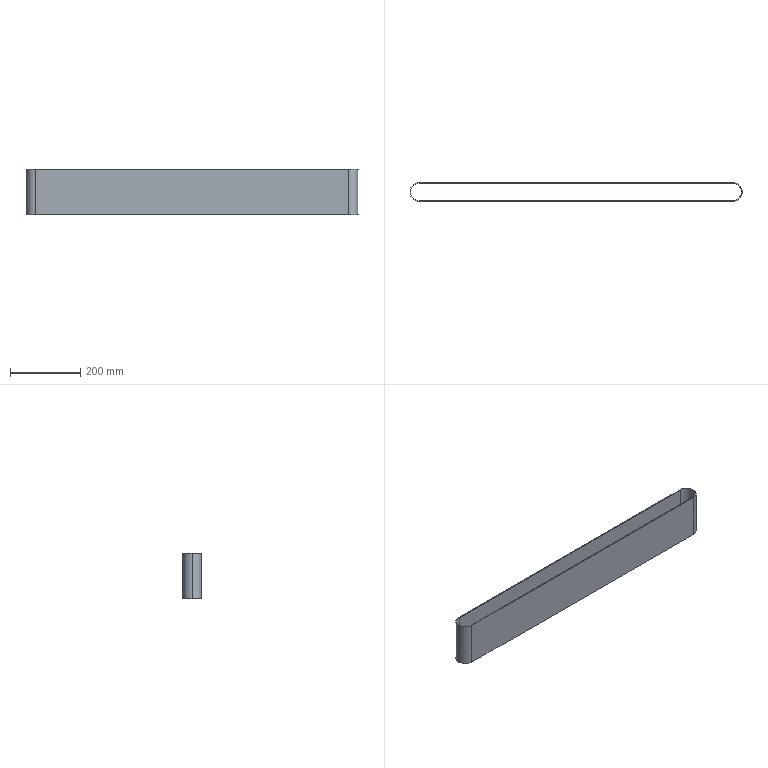Part | STEP file | Light green PVC conveyor belt 1946x129x2mm thick_antistatic | 1 solid | 12 faces | box 948.5 x 54 x 129 mm | volume 503710 mm3 | cylinder 6 | plane 6 | commonest cylinder face diameters 50 x3 54 x3
STEP:
#1=CARTESIAN_POINT('',(0.,0.,0.));
#2=DIRECTION('',(0.,0.,1.));
#3=DIRECTION('',(1.,0.,0.));
#4=AXIS2_PLACEMENT_3D('',#1,#2,#3);
#5=CARTESIAN_POINT('',(-447.25,25.,64.5));
#6=VERTEX_POINT('',#5);
#7=CARTESIAN_POINT('',(-447.25,25.,-64.5));
#8=VERTEX_POINT('',#7);
#9=CARTESIAN_POINT('',(-447.25,25.,64.5));
#10=DIRECTION('',(0.,0.,-1.));
#11=VECTOR('',#10,1.);
#12=LINE('',#9,#11);
#13=CARTESIAN_POINT('',(-447.25,0.,64.5));
#14=DIRECTION('',(0.,0.,-1.));
#15=DIRECTION('',(-1.,0.,0.));
#16=AXIS2_PLACEMENT_3D('',#13,#14,#15);
#17=CYLINDRICAL_SURFACE('',#16,25.);
#18=CARTESIAN_POINT('',(1.571,0.));
#19=DIRECTION('',(0.,1.));
#20=VECTOR('',#19,1.);
#21=LINE('',#18,#20);
#22=(GEOMETRIC_REPRESENTATION_CONTEXT(2)PARAMETRIC_REPRESENTATION_CONTEXT()REPRESENTATION_CONTEXT('',''));
#23=DEFINITIONAL_REPRESENTATION('',(#21),#22);
#24=PCURVE('',#17,#23);
#25=CARTESIAN_POINT('',(-447.25,25.,64.5));
#26=DIRECTION('',(0.,-1.,0.));
#27=DIRECTION('',(0.,0.,-1.));
#28=AXIS2_PLACEMENT_3D('',#25,#26,#27);
#29=PLANE('',#28);
#30=CARTESIAN_POINT('',(0.,0.));
#31=DIRECTION('',(1.,0.));
#32=VECTOR('',#31,1.);
#33=LINE('',#30,#32);
#34=(GEOMETRIC_REPRESENTATION_CONTEXT(2)PARAMETRIC_REPRESENTATION_CONTEXT()REPRESENTATION_CONTEXT('',''));
#35=DEFINITIONAL_REPRESENTATION('',(#33),#34);
#36=PCURVE('',#29,#35);
#37=SURFACE_CURVE('',#12,(#24,#36),.PCURVE_S1.);
#38=EDGE_CURVE('',#6,#8,#37,.T.);
#39=ORIENTED_EDGE('',*,*,#38,.T.);
#40=CARTESIAN_POINT('',(-472.25,0.,-64.5));
#41=VERTEX_POINT('',#40);
#42=CARTESIAN_POINT('',(-447.25,0.,-64.5));
#43=DIRECTION('',(0.,0.,1.));
#44=DIRECTION('',(1.,0.,0.));
#45=AXIS2_PLACEMENT_3D('',#42,#43,#44);
#46=CIRCLE('',#45,25.);
#47=CARTESIAN_POINT('',(3.142,129.));
#48=DIRECTION('',(-1.,0.));
#49=VECTOR('',#48,1.);
#50=LINE('',#47,#49);
#51=(GEOMETRIC_REPRESENTATION_CONTEXT(2)PARAMETRIC_REPRESENTATION_CONTEXT()REPRESENTATION_CONTEXT('',''));
#52=DEFINITIONAL_REPRESENTATION('',(#50),#51);
#53=PCURVE('',#17,#52);
#54=CARTESIAN_POINT('',(-447.25,0.,-64.5));
#55=DIRECTION('',(0.,0.,1.));
#56=DIRECTION('',(1.,0.,0.));
#57=AXIS2_PLACEMENT_3D('',#54,#55,#56);
#58=PLANE('',#57);
#59=CARTESIAN_POINT('',(0.,0.));
#60=DIRECTION('',(1.,0.));
#61=AXIS2_PLACEMENT_2D('',#59,#60);
#62=CIRCLE('',#61,25.);
#63=(GEOMETRIC_REPRESENTATION_CONTEXT(2)PARAMETRIC_REPRESENTATION_CONTEXT()REPRESENTATION_CONTEXT('',''));
#64=DEFINITIONAL_REPRESENTATION('',(#62),#63);
#65=PCURVE('',#58,#64);
#66=SURFACE_CURVE('',#46,(#53,#65),.PCURVE_S1.);
#67=EDGE_CURVE('',#8,#41,#66,.T.);
#68=ORIENTED_EDGE('',*,*,#67,.T.);
#69=CARTESIAN_POINT('',(-472.25,0.,64.5));
#70=VERTEX_POINT('',#69);
#71=CARTESIAN_POINT('',(-472.25,0.,64.5));
#72=DIRECTION('',(0.,0.,-1.));
#73=VECTOR('',#72,1.);
#74=LINE('',#71,#73);
#75=CARTESIAN_POINT('',(0.,0.));
#76=DIRECTION('',(0.,1.));
#77=VECTOR('',#76,1.);
#78=LINE('',#75,#77);
#79=(GEOMETRIC_REPRESENTATION_CONTEXT(2)PARAMETRIC_REPRESENTATION_CONTEXT()REPRESENTATION_CONTEXT('',''));
#80=DEFINITIONAL_REPRESENTATION('',(#78),#79);
#81=PCURVE('',#17,#80);
#82=CARTESIAN_POINT('',(-447.25,0.,64.5));
#83=DIRECTION('',(0.,0.,-1.));
#84=DIRECTION('',(-1.,0.,0.));
#85=AXIS2_PLACEMENT_3D('',#82,#83,#84);
#86=CYLINDRICAL_SURFACE('',#85,25.);
#87=CARTESIAN_POINT('',(6.283,0.));
#88=DIRECTION('',(0.,1.));
#89=VECTOR('',#88,1.);
#90=LINE('',#87,#89);
#91=(GEOMETRIC_REPRESENTATION_CONTEXT(2)PARAMETRIC_REPRESENTATION_CONTEXT()REPRESENTATION_CONTEXT('',''));
#92=DEFINITIONAL_REPRESENTATION('',(#90),#91);
#93=PCURVE('',#86,#92);
#94=SURFACE_CURVE('',#74,(#81,#93),.PCURVE_S1.);
#95=EDGE_CURVE('',#70,#41,#94,.T.);
#96=ORIENTED_EDGE('',*,*,#95,.F.);
#97=CARTESIAN_POINT('',(-447.25,0.,64.5));
#98=DIRECTION('',(0.,0.,1.));
#99=DIRECTION('',(1.,0.,0.));
#100=AXIS2_PLACEMENT_3D('',#97,#98,#99);
#101=CIRCLE('',#100,25.);
#102=CARTESIAN_POINT('',(3.142,0.));
#103=DIRECTION('',(-1.,0.));
#104=VECTOR('',#103,1.);
#105=LINE('',#102,#104);
#106=(GEOMETRIC_REPRESENTATION_CONTEXT(2)PARAMETRIC_REPRESENTATION_CONTEXT()REPRESENTATION_CONTEXT('',''));
#107=DEFINITIONAL_REPRESENTATION('',(#105),#106);
#108=PCURVE('',#17,#107);
#109=CARTESIAN_POINT('',(-447.25,0.,64.5));
#110=DIRECTION('',(0.,0.,1.));
#111=DIRECTION('',(1.,0.,0.));
#112=AXIS2_PLACEMENT_3D('',#109,#110,#111);
#113=PLANE('',#112);
#114=CARTESIAN_POINT('',(0.,0.));
#115=DIRECTION('',(1.,0.));
#116=AXIS2_PLACEMENT_2D('',#114,#115);
#117=CIRCLE('',#116,25.);
#118=(GEOMETRIC_REPRESENTATION_CONTEXT(2)PARAMETRIC_REPRESENTATION_CONTEXT()REPRESENTATION_CONTEXT('',''));
#119=DEFINITIONAL_REPRESENTATION('',(#117),#118);
#120=PCURVE('',#113,#119);
#121=SURFACE_CURVE('',#101,(#108,#120),.PCURVE_S1.);
#122=EDGE_CURVE('',#6,#70,#121,.T.);
#123=ORIENTED_EDGE('',*,*,#122,.F.);
#124=EDGE_LOOP('',(#39,#68,#96,#123));
#125=FACE_BOUND('',#124,.F.);
#126=ADVANCED_FACE('',(#125),#17,.F.);
#127=CARTESIAN_POINT('',(-474.25,0.,64.5));
#128=VERTEX_POINT('',#127);
#129=CARTESIAN_POINT('',(-447.25,-27.,64.5));
#130=VERTEX_POINT('',#129);
#131=CARTESIAN_POINT('',(-447.25,0.,64.5));
#132=DIRECTION('',(0.,0.,1.));
#133=DIRECTION('',(1.,0.,0.));
#134=AXIS2_PLACEMENT_3D('',#131,#132,#133);
#135=CIRCLE('',#134,27.);
#136=CARTESIAN_POINT('',(-447.25,0.,64.5));
#137=DIRECTION('',(0.,0.,-1.));
#138=DIRECTION('',(-1.,0.,0.));
#139=AXIS2_PLACEMENT_3D('',#136,#137,#138);
#140=CYLINDRICAL_SURFACE('',#139,27.);
#141=CARTESIAN_POINT('',(9.425,0.));
#142=DIRECTION('',(-1.,0.));
#143=VECTOR('',#142,1.);
#144=LINE('',#141,#143);
#145=(GEOMETRIC_REPRESENTATION_CONTEXT(2)PARAMETRIC_REPRESENTATION_CONTEXT()REPRESENTATION_CONTEXT('',''));
#146=DEFINITIONAL_REPRESENTATION('',(#144),#145);
#147=PCURVE('',#140,#146);
#148=CARTESIAN_POINT('',(0.,0.));
#149=DIRECTION('',(1.,0.));
#150=AXIS2_PLACEMENT_2D('',#148,#149);
#151=CIRCLE('',#150,27.);
#152=(GEOMETRIC_REPRESENTATION_CONTEXT(2)PARAMETRIC_REPRESENTATION_CONTEXT()REPRESENTATION_CONTEXT('',''));
#153=DEFINITIONAL_REPRESENTATION('',(#151),#152);
#154=PCURVE('',#113,#153);
#155=SURFACE_CURVE('',#135,(#147,#154),.PCURVE_S1.);
#156=EDGE_CURVE('',#128,#130,#155,.T.);
#157=ORIENTED_EDGE('',*,*,#156,.F.);
#158=CARTESIAN_POINT('',(-474.25,0.,-64.5));
#159=VERTEX_POINT('',#158);
#160=CARTESIAN_POINT('',(-474.25,0.,64.5));
#161=DIRECTION('',(0.,0.,-1.));
#162=VECTOR('',#161,1.);
#163=LINE('',#160,#162);
#164=CARTESIAN_POINT('',(6.283,0.));
#165=DIRECTION('',(0.,1.));
#166=VECTOR('',#165,1.);
#167=LINE('',#164,#166);
#168=(GEOMETRIC_REPRESENTATION_CONTEXT(2)PARAMETRIC_REPRESENTATION_CONTEXT()REPRESENTATION_CONTEXT('',''));
#169=DEFINITIONAL_REPRESENTATION('',(#167),#168);
#170=PCURVE('',#140,#169);
#171=CARTESIAN_POINT('',(-447.25,0.,64.5));
#172=DIRECTION('',(0.,0.,-1.));
#173=DIRECTION('',(-1.,0.,0.));
#174=AXIS2_PLACEMENT_3D('',#171,#172,#173);
#175=CYLINDRICAL_SURFACE('',#174,27.);
#176=CARTESIAN_POINT('',(0.,0.));
#177=DIRECTION('',(0.,1.));
#178=VECTOR('',#177,1.);
#179=LINE('',#176,#178);
#180=(GEOMETRIC_REPRESENTATION_CONTEXT(2)PARAMETRIC_REPRESENTATION_CONTEXT()REPRESENTATION_CONTEXT('',''));
#181=DEFINITIONAL_REPRESENTATION('',(#179),#180);
#182=PCURVE('',#175,#181);
#183=SURFACE_CURVE('',#163,(#170,#182),.PCURVE_S1.);
#184=EDGE_CURVE('',#128,#159,#183,.T.);
#185=ORIENTED_EDGE('',*,*,#184,.T.);
#186=CARTESIAN_POINT('',(-447.25,-27.,-64.5));
#187=VERTEX_POINT('',#186);
#188=CARTESIAN_POINT('',(-447.25,0.,-64.5));
#189=DIRECTION('',(0.,0.,1.));
#190=DIRECTION('',(1.,0.,0.));
#191=AXIS2_PLACEMENT_3D('',#188,#189,#190);
#192=CIRCLE('',#191,27.);
#193=CARTESIAN_POINT('',(9.425,129.));
#194=DIRECTION('',(-1.,0.));
#195=VECTOR('',#194,1.);
#196=LINE('',#193,#195);
#197=(GEOMETRIC_REPRESENTATION_CONTEXT(2)PARAMETRIC_REPRESENTATION_CONTEXT()REPRESENTATION_CONTEXT('',''));
#198=DEFINITIONAL_REPRESENTATION('',(#196),#197);
#199=PCURVE('',#140,#198);
#200=CARTESIAN_POINT('',(0.,0.));
#201=DIRECTION('',(1.,0.));
#202=AXIS2_PLACEMENT_2D('',#200,#201);
#203=CIRCLE('',#202,27.);
#204=(GEOMETRIC_REPRESENTATION_CONTEXT(2)PARAMETRIC_REPRESENTATION_CONTEXT()REPRESENTATION_CONTEXT('',''));
#205=DEFINITIONAL_REPRESENTATION('',(#203),#204);
#206=PCURVE('',#58,#205);
#207=SURFACE_CURVE('',#192,(#199,#206),.PCURVE_S1.);
#208=EDGE_CURVE('',#159,#187,#207,.T.);
#209=ORIENTED_EDGE('',*,*,#208,.T.);
#210=CARTESIAN_POINT('',(-447.25,-27.,64.5));
#211=DIRECTION('',(0.,0.,-1.));
#212=VECTOR('',#211,1.);
#213=LINE('',#210,#212);
#214=CARTESIAN_POINT('',(4.712,0.));
#215=DIRECTION('',(0.,1.));
#216=VECTOR('',#215,1.);
#217=LINE('',#214,#216);
#218=(GEOMETRIC_REPRESENTATION_CONTEXT(2)PARAMETRIC_REPRESENTATION_CONTEXT()REPRESENTATION_CONTEXT('',''));
#219=DEFINITIONAL_REPRESENTATION('',(#217),#218);
#220=PCURVE('',#140,#219);
#221=CARTESIAN_POINT('',(-447.25,-27.,64.5));
#222=DIRECTION('',(0.,1.,0.));
#223=DIRECTION('',(0.,0.,1.));
#224=AXIS2_PLACEMENT_3D('',#221,#222,#223);
#225=PLANE('',#224);
#226=CARTESIAN_POINT('',(0.,0.));
#227=DIRECTION('',(-1.,0.));
#228=VECTOR('',#227,1.);
#229=LINE('',#226,#228);
#230=(GEOMETRIC_REPRESENTATION_CONTEXT(2)PARAMETRIC_REPRESENTATION_CONTEXT()REPRESENTATION_CONTEXT('',''));
#231=DEFINITIONAL_REPRESENTATION('',(#229),#230);
#232=PCURVE('',#225,#231);
#233=SURFACE_CURVE('',#213,(#220,#232),.PCURVE_S1.);
#234=EDGE_CURVE('',#130,#187,#233,.T.);
#235=ORIENTED_EDGE('',*,*,#234,.F.);
#236=EDGE_LOOP('',(#157,#185,#209,#235));
#237=FACE_BOUND('',#236,.T.);
#238=ADVANCED_FACE('',(#237),#140,.T.);
#239=CARTESIAN_POINT('',(-447.25,27.,64.5));
#240=VERTEX_POINT('',#239);
#241=CARTESIAN_POINT('',(-447.25,0.,64.5));
#242=DIRECTION('',(0.,0.,1.));
#243=DIRECTION('',(1.,0.,0.));
#244=AXIS2_PLACEMENT_3D('',#241,#242,#243);
#245=CIRCLE('',#244,27.);
#246=CARTESIAN_POINT('',(0.,0.));
#247=DIRECTION('',(1.,0.));
#248=AXIS2_PLACEMENT_2D('',#246,#247);
#249=CIRCLE('',#248,27.);
#250=(GEOMETRIC_REPRESENTATION_CONTEXT(2)PARAMETRIC_REPRESENTATION_CONTEXT()REPRESENTATION_CONTEXT('',''));
#251=DEFINITIONAL_REPRESENTATION('',(#249),#250);
#252=PCURVE('',#113,#251);
#253=CARTESIAN_POINT('',(3.142,0.));
#254=DIRECTION('',(-1.,0.));
#255=VECTOR('',#254,1.);
#256=LINE('',#253,#255);
#257=(GEOMETRIC_REPRESENTATION_CONTEXT(2)PARAMETRIC_REPRESENTATION_CONTEXT()REPRESENTATION_CONTEXT('',''));
#258=DEFINITIONAL_REPRESENTATION('',(#256),#257);
#259=PCURVE('',#175,#258);
#260=SURFACE_CURVE('',#245,(#252,#259),.PCURVE_S1.);
#261=EDGE_CURVE('',#240,#128,#260,.T.);
#262=ORIENTED_EDGE('',*,*,#261,.T.);
#263=ORIENTED_EDGE('',*,*,#156,.T.);
#264=CARTESIAN_POINT('',(447.25,-27.,64.5));
#265=VERTEX_POINT('',#264);
#266=CARTESIAN_POINT('',(-447.25,-27.,64.5));
#267=DIRECTION('',(1.,0.,0.));
#268=VECTOR('',#267,1.);
#269=LINE('',#266,#268);
#270=CARTESIAN_POINT('',(0.,-27.));
#271=DIRECTION('',(1.,0.));
#272=VECTOR('',#271,1.);
#273=LINE('',#270,#272);
#274=(GEOMETRIC_REPRESENTATION_CONTEXT(2)PARAMETRIC_REPRESENTATION_CONTEXT()REPRESENTATION_CONTEXT('',''));
#275=DEFINITIONAL_REPRESENTATION('',(#273),#274);
#276=PCURVE('',#113,#275);
#277=CARTESIAN_POINT('',(0.,0.));
#278=DIRECTION('',(0.,1.));
#279=VECTOR('',#278,1.);
#280=LINE('',#277,#279);
#281=(GEOMETRIC_REPRESENTATION_CONTEXT(2)PARAMETRIC_REPRESENTATION_CONTEXT()REPRESENTATION_CONTEXT('',''));
#282=DEFINITIONAL_REPRESENTATION('',(#280),#281);
#283=PCURVE('',#225,#282);
#284=SURFACE_CURVE('',#269,(#276,#283),.PCURVE_S1.);
#285=EDGE_CURVE('',#130,#265,#284,.T.);
#286=ORIENTED_EDGE('',*,*,#285,.T.);
#287=CARTESIAN_POINT('',(447.25,27.,64.5));
#288=VERTEX_POINT('',#287);
#289=CARTESIAN_POINT('',(447.25,0.,64.5));
#290=DIRECTION('',(0.,0.,1.));
#291=DIRECTION('',(1.,0.,0.));
#292=AXIS2_PLACEMENT_3D('',#289,#290,#291);
#293=CIRCLE('',#292,27.);
#294=CARTESIAN_POINT('',(894.5,0.));
#295=DIRECTION('',(1.,0.));
#296=AXIS2_PLACEMENT_2D('',#294,#295);
#297=CIRCLE('',#296,27.);
#298=(GEOMETRIC_REPRESENTATION_CONTEXT(2)PARAMETRIC_REPRESENTATION_CONTEXT()REPRESENTATION_CONTEXT('',''));
#299=DEFINITIONAL_REPRESENTATION('',(#297),#298);
#300=PCURVE('',#113,#299);
#301=CARTESIAN_POINT('',(447.25,0.,64.5));
#302=DIRECTION('',(0.,0.,-1.));
#303=DIRECTION('',(-1.,0.,0.));
#304=AXIS2_PLACEMENT_3D('',#301,#302,#303);
#305=CYLINDRICAL_SURFACE('',#304,27.);
#306=CARTESIAN_POINT('',(9.425,0.));
#307=DIRECTION('',(-1.,0.));
#308=VECTOR('',#307,1.);
#309=LINE('',#306,#308);
#310=(GEOMETRIC_REPRESENTATION_CONTEXT(2)PARAMETRIC_REPRESENTATION_CONTEXT()REPRESENTATION_CONTEXT('',''));
#311=DEFINITIONAL_REPRESENTATION('',(#309),#310);
#312=PCURVE('',#305,#311);
#313=SURFACE_CURVE('',#293,(#300,#312),.PCURVE_S1.);
#314=EDGE_CURVE('',#265,#288,#313,.T.);
#315=ORIENTED_EDGE('',*,*,#314,.T.);
#316=CARTESIAN_POINT('',(-447.25,27.,64.5));
#317=DIRECTION('',(-1.,0.,0.));
#318=VECTOR('',#317,1.);
#319=LINE('',#316,#318);
#320=CARTESIAN_POINT('',(0.,27.));
#321=DIRECTION('',(-1.,0.));
#322=VECTOR('',#321,1.);
#323=LINE('',#320,#322);
#324=(GEOMETRIC_REPRESENTATION_CONTEXT(2)PARAMETRIC_REPRESENTATION_CONTEXT()REPRESENTATION_CONTEXT('',''));
#325=DEFINITIONAL_REPRESENTATION('',(#323),#324);
#326=PCURVE('',#113,#325);
#327=CARTESIAN_POINT('',(-447.25,27.,64.5));
#328=DIRECTION('',(0.,-1.,0.));
#329=DIRECTION('',(0.,0.,-1.));
#330=AXIS2_PLACEMENT_3D('',#327,#328,#329);
#331=PLANE('',#330);
#332=CARTESIAN_POINT('',(0.,0.));
#333=DIRECTION('',(0.,-1.));
#334=VECTOR('',#333,1.);
#335=LINE('',#332,#334);
#336=(GEOMETRIC_REPRESENTATION_CONTEXT(2)PARAMETRIC_REPRESENTATION_CONTEXT()REPRESENTATION_CONTEXT('',''));
#337=DEFINITIONAL_REPRESENTATION('',(#335),#336);
#338=PCURVE('',#331,#337);
#339=SURFACE_CURVE('',#319,(#326,#338),.PCURVE_S1.);
#340=EDGE_CURVE('',#288,#240,#339,.T.);
#341=ORIENTED_EDGE('',*,*,#340,.T.);
#342=EDGE_LOOP('',(#262,#263,#286,#315,#341));
#343=FACE_BOUND('',#342,.T.);
#344=CARTESIAN_POINT('',(-447.25,-25.,64.5));
#345=VERTEX_POINT('',#344);
#346=CARTESIAN_POINT('',(447.25,-25.,64.5));
#347=VERTEX_POINT('',#346);
#348=CARTESIAN_POINT('',(-447.25,-25.,64.5));
#349=DIRECTION('',(1.,0.,0.));
#350=VECTOR('',#349,1.);
#351=LINE('',#348,#350);
#352=CARTESIAN_POINT('',(0.,-25.));
#353=DIRECTION('',(1.,0.));
#354=VECTOR('',#353,1.);
#355=LINE('',#352,#354);
#356=(GEOMETRIC_REPRESENTATION_CONTEXT(2)PARAMETRIC_REPRESENTATION_CONTEXT()REPRESENTATION_CONTEXT('',''));
#357=DEFINITIONAL_REPRESENTATION('',(#355),#356);
#358=PCURVE('',#113,#357);
#359=CARTESIAN_POINT('',(-447.25,-25.,64.5));
#360=DIRECTION('',(0.,1.,0.));
#361=DIRECTION('',(0.,0.,1.));
#362=AXIS2_PLACEMENT_3D('',#359,#360,#361);
#363=PLANE('',#362);
#364=CARTESIAN_POINT('',(0.,0.));
#365=DIRECTION('',(0.,1.));
#366=VECTOR('',#365,1.);
#367=LINE('',#364,#366);
#368=(GEOMETRIC_REPRESENTATION_CONTEXT(2)PARAMETRIC_REPRESENTATION_CONTEXT()REPRESENTATION_CONTEXT('',''));
#369=DEFINITIONAL_REPRESENTATION('',(#367),#368);
#370=PCURVE('',#363,#369);
#371=SURFACE_CURVE('',#351,(#358,#370),.PCURVE_S1.);
#372=EDGE_CURVE('',#345,#347,#371,.T.);
#373=ORIENTED_EDGE('',*,*,#372,.F.);
#374=CARTESIAN_POINT('',(-447.25,0.,64.5));
#375=DIRECTION('',(0.,0.,1.));
#376=DIRECTION('',(1.,0.,0.));
#377=AXIS2_PLACEMENT_3D('',#374,#375,#376);
#378=CIRCLE('',#377,25.);
#379=CARTESIAN_POINT('',(0.,0.));
#380=DIRECTION('',(1.,0.));
#381=AXIS2_PLACEMENT_2D('',#379,#380);
#382=CIRCLE('',#381,25.);
#383=(GEOMETRIC_REPRESENTATION_CONTEXT(2)PARAMETRIC_REPRESENTATION_CONTEXT()REPRESENTATION_CONTEXT('',''));
#384=DEFINITIONAL_REPRESENTATION('',(#382),#383);
#385=PCURVE('',#113,#384);
#386=CARTESIAN_POINT('',(9.425,0.));
#387=DIRECTION('',(-1.,0.));
#388=VECTOR('',#387,1.);
#389=LINE('',#386,#388);
#390=(GEOMETRIC_REPRESENTATION_CONTEXT(2)PARAMETRIC_REPRESENTATION_CONTEXT()REPRESENTATION_CONTEXT('',''));
#391=DEFINITIONAL_REPRESENTATION('',(#389),#390);
#392=PCURVE('',#86,#391);
#393=SURFACE_CURVE('',#378,(#385,#392),.PCURVE_S1.);
#394=EDGE_CURVE('',#70,#345,#393,.T.);
#395=ORIENTED_EDGE('',*,*,#394,.F.);
#396=ORIENTED_EDGE('',*,*,#122,.F.);
#397=CARTESIAN_POINT('',(447.25,25.,64.5));
#398=VERTEX_POINT('',#397);
#399=CARTESIAN_POINT('',(-447.25,25.,64.5));
#400=DIRECTION('',(-1.,0.,0.));
#401=VECTOR('',#400,1.);
#402=LINE('',#399,#401);
#403=CARTESIAN_POINT('',(0.,25.));
#404=DIRECTION('',(-1.,0.));
#405=VECTOR('',#404,1.);
#406=LINE('',#403,#405);
#407=(GEOMETRIC_REPRESENTATION_CONTEXT(2)PARAMETRIC_REPRESENTATION_CONTEXT()REPRESENTATION_CONTEXT('',''));
#408=DEFINITIONAL_REPRESENTATION('',(#406),#407);
#409=PCURVE('',#113,#408);
#410=CARTESIAN_POINT('',(0.,0.));
#411=DIRECTION('',(0.,-1.));
#412=VECTOR('',#411,1.);
#413=LINE('',#410,#412);
#414=(GEOMETRIC_REPRESENTATION_CONTEXT(2)PARAMETRIC_REPRESENTATION_CONTEXT()REPRESENTATION_CONTEXT('',''));
#415=DEFINITIONAL_REPRESENTATION('',(#413),#414);
#416=PCURVE('',#29,#415);
#417=SURFACE_CURVE('',#402,(#409,#416),.PCURVE_S1.);
#418=EDGE_CURVE('',#398,#6,#417,.T.);
#419=ORIENTED_EDGE('',*,*,#418,.F.);
#420=CARTESIAN_POINT('',(447.25,0.,64.5));
#421=DIRECTION('',(0.,0.,1.));
#422=DIRECTION('',(1.,0.,0.));
#423=AXIS2_PLACEMENT_3D('',#420,#421,#422);
#424=CIRCLE('',#423,25.);
#425=CARTESIAN_POINT('',(894.5,0.));
#426=DIRECTION('',(1.,0.));
#427=AXIS2_PLACEMENT_2D('',#425,#426);
#428=CIRCLE('',#427,25.);
#429=(GEOMETRIC_REPRESENTATION_CONTEXT(2)PARAMETRIC_REPRESENTATION_CONTEXT()REPRESENTATION_CONTEXT('',''));
#430=DEFINITIONAL_REPRESENTATION('',(#428),#429);
#431=PCURVE('',#113,#430);
#432=CARTESIAN_POINT('',(447.25,0.,64.5));
#433=DIRECTION('',(0.,0.,-1.));
#434=DIRECTION('',(-1.,0.,0.));
#435=AXIS2_PLACEMENT_3D('',#432,#433,#434);
#436=CYLINDRICAL_SURFACE('',#435,25.);
#437=CARTESIAN_POINT('',(9.425,0.));
#438=DIRECTION('',(-1.,0.));
#439=VECTOR('',#438,1.);
#440=LINE('',#437,#439);
#441=(GEOMETRIC_REPRESENTATION_CONTEXT(2)PARAMETRIC_REPRESENTATION_CONTEXT()REPRESENTATION_CONTEXT('',''));
#442=DEFINITIONAL_REPRESENTATION('',(#440),#441);
#443=PCURVE('',#436,#442);
#444=SURFACE_CURVE('',#424,(#431,#443),.PCURVE_S1.);
#445=EDGE_CURVE('',#347,#398,#444,.T.);
#446=ORIENTED_EDGE('',*,*,#445,.F.);
#447=EDGE_LOOP('',(#373,#395,#396,#419,#446));
#448=FACE_BOUND('',#447,.T.);
#449=ADVANCED_FACE('',(#343,#448),#113,.T.);
#450=CARTESIAN_POINT('',(-447.25,27.,-64.5));
#451=VERTEX_POINT('',#450);
#452=CARTESIAN_POINT('',(-447.25,0.,-64.5));
#453=DIRECTION('',(0.,0.,1.));
#454=DIRECTION('',(1.,0.,0.));
#455=AXIS2_PLACEMENT_3D('',#452,#453,#454);
#456=CIRCLE('',#455,27.);
#457=CARTESIAN_POINT('',(0.,0.));
#458=DIRECTION('',(1.,0.));
#459=AXIS2_PLACEMENT_2D('',#457,#458);
#460=CIRCLE('',#459,27.);
#461=(GEOMETRIC_REPRESENTATION_CONTEXT(2)PARAMETRIC_REPRESENTATION_CONTEXT()REPRESENTATION_CONTEXT('',''));
#462=DEFINITIONAL_REPRESENTATION('',(#460),#461);
#463=PCURVE('',#58,#462);
#464=CARTESIAN_POINT('',(3.142,129.));
#465=DIRECTION('',(-1.,0.));
#466=VECTOR('',#465,1.);
#467=LINE('',#464,#466);
#468=(GEOMETRIC_REPRESENTATION_CONTEXT(2)PARAMETRIC_REPRESENTATION_CONTEXT()REPRESENTATION_CONTEXT('',''));
#469=DEFINITIONAL_REPRESENTATION('',(#467),#468);
#470=PCURVE('',#175,#469);
#471=SURFACE_CURVE('',#456,(#463,#470),.PCURVE_S1.);
#472=EDGE_CURVE('',#451,#159,#471,.T.);
#473=ORIENTED_EDGE('',*,*,#472,.F.);
#474=CARTESIAN_POINT('',(447.25,27.,-64.5));
#475=VERTEX_POINT('',#474);
#476=CARTESIAN_POINT('',(-447.25,27.,-64.5));
#477=DIRECTION('',(-1.,0.,0.));
#478=VECTOR('',#477,1.);
#479=LINE('',#476,#478);
#480=CARTESIAN_POINT('',(0.,27.));
#481=DIRECTION('',(-1.,0.));
#482=VECTOR('',#481,1.);
#483=LINE('',#480,#482);
#484=(GEOMETRIC_REPRESENTATION_CONTEXT(2)PARAMETRIC_REPRESENTATION_CONTEXT()REPRESENTATION_CONTEXT('',''));
#485=DEFINITIONAL_REPRESENTATION('',(#483),#484);
#486=PCURVE('',#58,#485);
#487=CARTESIAN_POINT('',(129.,0.));
#488=DIRECTION('',(0.,-1.));
#489=VECTOR('',#488,1.);
#490=LINE('',#487,#489);
#491=(GEOMETRIC_REPRESENTATION_CONTEXT(2)PARAMETRIC_REPRESENTATION_CONTEXT()REPRESENTATION_CONTEXT('',''));
#492=DEFINITIONAL_REPRESENTATION('',(#490),#491);
#493=PCURVE('',#331,#492);
#494=SURFACE_CURVE('',#479,(#486,#493),.PCURVE_S1.);
#495=EDGE_CURVE('',#475,#451,#494,.T.);
#496=ORIENTED_EDGE('',*,*,#495,.F.);
#497=CARTESIAN_POINT('',(447.25,-27.,-64.5));
#498=VERTEX_POINT('',#497);
#499=CARTESIAN_POINT('',(447.25,0.,-64.5));
#500=DIRECTION('',(0.,0.,1.));
#501=DIRECTION('',(1.,0.,0.));
#502=AXIS2_PLACEMENT_3D('',#499,#500,#501);
#503=CIRCLE('',#502,27.);
#504=CARTESIAN_POINT('',(894.5,0.));
#505=DIRECTION('',(1.,0.));
#506=AXIS2_PLACEMENT_2D('',#504,#505);
#507=CIRCLE('',#506,27.);
#508=(GEOMETRIC_REPRESENTATION_CONTEXT(2)PARAMETRIC_REPRESENTATION_CONTEXT()REPRESENTATION_CONTEXT('',''));
#509=DEFINITIONAL_REPRESENTATION('',(#507),#508);
#510=PCURVE('',#58,#509);
#511=CARTESIAN_POINT('',(9.425,129.));
#512=DIRECTION('',(-1.,0.));
#513=VECTOR('',#512,1.);
#514=LINE('',#511,#513);
#515=(GEOMETRIC_REPRESENTATION_CONTEXT(2)PARAMETRIC_REPRESENTATION_CONTEXT()REPRESENTATION_CONTEXT('',''));
#516=DEFINITIONAL_REPRESENTATION('',(#514),#515);
#517=PCURVE('',#305,#516);
#518=SURFACE_CURVE('',#503,(#510,#517),.PCURVE_S1.);
#519=EDGE_CURVE('',#498,#475,#518,.T.);
#520=ORIENTED_EDGE('',*,*,#519,.F.);
#521=CARTESIAN_POINT('',(-447.25,-27.,-64.5));
#522=DIRECTION('',(1.,0.,0.));
#523=VECTOR('',#522,1.);
#524=LINE('',#521,#523);
#525=CARTESIAN_POINT('',(0.,-27.));
#526=DIRECTION('',(1.,0.));
#527=VECTOR('',#526,1.);
#528=LINE('',#525,#527);
#529=(GEOMETRIC_REPRESENTATION_CONTEXT(2)PARAMETRIC_REPRESENTATION_CONTEXT()REPRESENTATION_CONTEXT('',''));
#530=DEFINITIONAL_REPRESENTATION('',(#528),#529);
#531=PCURVE('',#58,#530);
#532=CARTESIAN_POINT('',(-129.,0.));
#533=DIRECTION('',(0.,1.));
#534=VECTOR('',#533,1.);
#535=LINE('',#532,#534);
#536=(GEOMETRIC_REPRESENTATION_CONTEXT(2)PARAMETRIC_REPRESENTATION_CONTEXT()REPRESENTATION_CONTEXT('',''));
#537=DEFINITIONAL_REPRESENTATION('',(#535),#536);
#538=PCURVE('',#225,#537);
#539=SURFACE_CURVE('',#524,(#531,#538),.PCURVE_S1.);
#540=EDGE_CURVE('',#187,#498,#539,.T.);
#541=ORIENTED_EDGE('',*,*,#540,.F.);
#542=ORIENTED_EDGE('',*,*,#208,.F.);
#543=EDGE_LOOP('',(#473,#496,#520,#541,#542));
#544=FACE_BOUND('',#543,.T.);
#545=ORIENTED_EDGE('',*,*,#67,.T.);
#546=CARTESIAN_POINT('',(-447.25,-25.,-64.5));
#547=VERTEX_POINT('',#546);
#548=CARTESIAN_POINT('',(-447.25,0.,-64.5));
#549=DIRECTION('',(0.,0.,1.));
#550=DIRECTION('',(1.,0.,0.));
#551=AXIS2_PLACEMENT_3D('',#548,#549,#550);
#552=CIRCLE('',#551,25.);
#553=CARTESIAN_POINT('',(0.,0.));
#554=DIRECTION('',(1.,0.));
#555=AXIS2_PLACEMENT_2D('',#553,#554);
#556=CIRCLE('',#555,25.);
#557=(GEOMETRIC_REPRESENTATION_CONTEXT(2)PARAMETRIC_REPRESENTATION_CONTEXT()REPRESENTATION_CONTEXT('',''));
#558=DEFINITIONAL_REPRESENTATION('',(#556),#557);
#559=PCURVE('',#58,#558);
#560=CARTESIAN_POINT('',(9.425,129.));
#561=DIRECTION('',(-1.,0.));
#562=VECTOR('',#561,1.);
#563=LINE('',#560,#562);
#564=(GEOMETRIC_REPRESENTATION_CONTEXT(2)PARAMETRIC_REPRESENTATION_CONTEXT()REPRESENTATION_CONTEXT('',''));
#565=DEFINITIONAL_REPRESENTATION('',(#563),#564);
#566=PCURVE('',#86,#565);
#567=SURFACE_CURVE('',#552,(#559,#566),.PCURVE_S1.);
#568=EDGE_CURVE('',#41,#547,#567,.T.);
#569=ORIENTED_EDGE('',*,*,#568,.T.);
#570=CARTESIAN_POINT('',(447.25,-25.,-64.5));
#571=VERTEX_POINT('',#570);
#572=CARTESIAN_POINT('',(-447.25,-25.,-64.5));
#573=DIRECTION('',(1.,0.,0.));
#574=VECTOR('',#573,1.);
#575=LINE('',#572,#574);
#576=CARTESIAN_POINT('',(0.,-25.));
#577=DIRECTION('',(1.,0.));
#578=VECTOR('',#577,1.);
#579=LINE('',#576,#578);
#580=(GEOMETRIC_REPRESENTATION_CONTEXT(2)PARAMETRIC_REPRESENTATION_CONTEXT()REPRESENTATION_CONTEXT('',''));
#581=DEFINITIONAL_REPRESENTATION('',(#579),#580);
#582=PCURVE('',#58,#581);
#583=CARTESIAN_POINT('',(-129.,0.));
#584=DIRECTION('',(0.,1.));
#585=VECTOR('',#584,1.);
#586=LINE('',#583,#585);
#587=(GEOMETRIC_REPRESENTATION_CONTEXT(2)PARAMETRIC_REPRESENTATION_CONTEXT()REPRESENTATION_CONTEXT('',''));
#588=DEFINITIONAL_REPRESENTATION('',(#586),#587);
#589=PCURVE('',#363,#588);
#590=SURFACE_CURVE('',#575,(#582,#589),.PCURVE_S1.);
#591=EDGE_CURVE('',#547,#571,#590,.T.);
#592=ORIENTED_EDGE('',*,*,#591,.T.);
#593=CARTESIAN_POINT('',(447.25,25.,-64.5));
#594=VERTEX_POINT('',#593);
#595=CARTESIAN_POINT('',(447.25,0.,-64.5));
#596=DIRECTION('',(0.,0.,1.));
#597=DIRECTION('',(1.,0.,0.));
#598=AXIS2_PLACEMENT_3D('',#595,#596,#597);
#599=CIRCLE('',#598,25.);
#600=CARTESIAN_POINT('',(894.5,0.));
#601=DIRECTION('',(1.,0.));
#602=AXIS2_PLACEMENT_2D('',#600,#601);
#603=CIRCLE('',#602,25.);
#604=(GEOMETRIC_REPRESENTATION_CONTEXT(2)PARAMETRIC_REPRESENTATION_CONTEXT()REPRESENTATION_CONTEXT('',''));
#605=DEFINITIONAL_REPRESENTATION('',(#603),#604);
#606=PCURVE('',#58,#605);
#607=CARTESIAN_POINT('',(9.425,129.));
#608=DIRECTION('',(-1.,0.));
#609=VECTOR('',#608,1.);
#610=LINE('',#607,#609);
#611=(GEOMETRIC_REPRESENTATION_CONTEXT(2)PARAMETRIC_REPRESENTATION_CONTEXT()REPRESENTATION_CONTEXT('',''));
#612=DEFINITIONAL_REPRESENTATION('',(#610),#611);
#613=PCURVE('',#436,#612);
#614=SURFACE_CURVE('',#599,(#606,#613),.PCURVE_S1.);
#615=EDGE_CURVE('',#571,#594,#614,.T.);
#616=ORIENTED_EDGE('',*,*,#615,.T.);
#617=CARTESIAN_POINT('',(-447.25,25.,-64.5));
#618=DIRECTION('',(-1.,0.,0.));
#619=VECTOR('',#618,1.);
#620=LINE('',#617,#619);
#621=CARTESIAN_POINT('',(0.,25.));
#622=DIRECTION('',(-1.,0.));
#623=VECTOR('',#622,1.);
#624=LINE('',#621,#623);
#625=(GEOMETRIC_REPRESENTATION_CONTEXT(2)PARAMETRIC_REPRESENTATION_CONTEXT()REPRESENTATION_CONTEXT('',''));
#626=DEFINITIONAL_REPRESENTATION('',(#624),#625);
#627=PCURVE('',#58,#626);
#628=CARTESIAN_POINT('',(129.,0.));
#629=DIRECTION('',(0.,-1.));
#630=VECTOR('',#629,1.);
#631=LINE('',#628,#630);
#632=(GEOMETRIC_REPRESENTATION_CONTEXT(2)PARAMETRIC_REPRESENTATION_CONTEXT()REPRESENTATION_CONTEXT('',''));
#633=DEFINITIONAL_REPRESENTATION('',(#631),#632);
#634=PCURVE('',#29,#633);
#635=SURFACE_CURVE('',#620,(#627,#634),.PCURVE_S1.);
#636=EDGE_CURVE('',#594,#8,#635,.T.);
#637=ORIENTED_EDGE('',*,*,#636,.T.);
#638=EDGE_LOOP('',(#545,#569,#592,#616,#637));
#639=FACE_BOUND('',#638,.T.);
#640=ADVANCED_FACE('',(#544,#639),#58,.F.);
#641=ORIENTED_EDGE('',*,*,#184,.F.);
#642=ORIENTED_EDGE('',*,*,#261,.F.);
#643=CARTESIAN_POINT('',(-447.25,27.,64.5));
#644=DIRECTION('',(0.,0.,-1.));
#645=VECTOR('',#644,1.);
#646=LINE('',#643,#645);
#647=CARTESIAN_POINT('',(1.571,0.));
#648=DIRECTION('',(0.,1.));
#649=VECTOR('',#648,1.);
#650=LINE('',#647,#649);
#651=(GEOMETRIC_REPRESENTATION_CONTEXT(2)PARAMETRIC_REPRESENTATION_CONTEXT()REPRESENTATION_CONTEXT('',''));
#652=DEFINITIONAL_REPRESENTATION('',(#650),#651);
#653=PCURVE('',#175,#652);
#654=CARTESIAN_POINT('',(0.,0.));
#655=DIRECTION('',(1.,0.));
#656=VECTOR('',#655,1.);
#657=LINE('',#654,#656);
#658=(GEOMETRIC_REPRESENTATION_CONTEXT(2)PARAMETRIC_REPRESENTATION_CONTEXT()REPRESENTATION_CONTEXT('',''));
#659=DEFINITIONAL_REPRESENTATION('',(#657),#658);
#660=PCURVE('',#331,#659);
#661=SURFACE_CURVE('',#646,(#653,#660),.PCURVE_S1.);
#662=EDGE_CURVE('',#240,#451,#661,.T.);
#663=ORIENTED_EDGE('',*,*,#662,.T.);
#664=ORIENTED_EDGE('',*,*,#472,.T.);
#665=EDGE_LOOP('',(#641,#642,#663,#664));
#666=FACE_BOUND('',#665,.T.);
#667=ADVANCED_FACE('',(#666),#175,.T.);
#668=ORIENTED_EDGE('',*,*,#540,.T.);
#669=CARTESIAN_POINT('',(447.25,-27.,64.5));
#670=DIRECTION('',(0.,0.,-1.));
#671=VECTOR('',#670,1.);
#672=LINE('',#669,#671);
#673=CARTESIAN_POINT('',(0.,894.5));
#674=DIRECTION('',(-1.,0.));
#675=VECTOR('',#674,1.);
#676=LINE('',#673,#675);
#677=(GEOMETRIC_REPRESENTATION_CONTEXT(2)PARAMETRIC_REPRESENTATION_CONTEXT()REPRESENTATION_CONTEXT('',''));
#678=DEFINITIONAL_REPRESENTATION('',(#676),#677);
#679=PCURVE('',#225,#678);
#680=CARTESIAN_POINT('',(4.712,0.));
#681=DIRECTION('',(0.,1.));
#682=VECTOR('',#681,1.);
#683=LINE('',#680,#682);
#684=(GEOMETRIC_REPRESENTATION_CONTEXT(2)PARAMETRIC_REPRESENTATION_CONTEXT()REPRESENTATION_CONTEXT('',''));
#685=DEFINITIONAL_REPRESENTATION('',(#683),#684);
#686=PCURVE('',#305,#685);
#687=SURFACE_CURVE('',#672,(#679,#686),.PCURVE_S1.);
#688=EDGE_CURVE('',#265,#498,#687,.T.);
#689=ORIENTED_EDGE('',*,*,#688,.F.);
#690=ORIENTED_EDGE('',*,*,#285,.F.);
#691=ORIENTED_EDGE('',*,*,#234,.T.);
#692=EDGE_LOOP('',(#668,#689,#690,#691));
#693=FACE_BOUND('',#692,.T.);
#694=ADVANCED_FACE('',(#693),#225,.F.);
#695=ORIENTED_EDGE('',*,*,#519,.T.);
#696=CARTESIAN_POINT('',(447.25,27.,64.5));
#697=DIRECTION('',(0.,0.,-1.));
#698=VECTOR('',#697,1.);
#699=LINE('',#696,#698);
#700=CARTESIAN_POINT('',(1.571,0.));
#701=DIRECTION('',(0.,1.));
#702=VECTOR('',#701,1.);
#703=LINE('',#700,#702);
#704=(GEOMETRIC_REPRESENTATION_CONTEXT(2)PARAMETRIC_REPRESENTATION_CONTEXT()REPRESENTATION_CONTEXT('',''));
#705=DEFINITIONAL_REPRESENTATION('',(#703),#704);
#706=PCURVE('',#305,#705);
#707=CARTESIAN_POINT('',(0.,894.5));
#708=DIRECTION('',(1.,0.));
#709=VECTOR('',#708,1.);
#710=LINE('',#707,#709);
#711=(GEOMETRIC_REPRESENTATION_CONTEXT(2)PARAMETRIC_REPRESENTATION_CONTEXT()REPRESENTATION_CONTEXT('',''));
#712=DEFINITIONAL_REPRESENTATION('',(#710),#711);
#713=PCURVE('',#331,#712);
#714=SURFACE_CURVE('',#699,(#706,#713),.PCURVE_S1.);
#715=EDGE_CURVE('',#288,#475,#714,.T.);
#716=ORIENTED_EDGE('',*,*,#715,.F.);
#717=ORIENTED_EDGE('',*,*,#314,.F.);
#718=ORIENTED_EDGE('',*,*,#688,.T.);
#719=EDGE_LOOP('',(#695,#716,#717,#718));
#720=FACE_BOUND('',#719,.T.);
#721=ADVANCED_FACE('',(#720),#305,.T.);
#722=ORIENTED_EDGE('',*,*,#495,.T.);
#723=ORIENTED_EDGE('',*,*,#662,.F.);
#724=ORIENTED_EDGE('',*,*,#340,.F.);
#725=ORIENTED_EDGE('',*,*,#715,.T.);
#726=EDGE_LOOP('',(#722,#723,#724,#725));
#727=FACE_BOUND('',#726,.T.);
#728=ADVANCED_FACE('',(#727),#331,.F.);
#729=ORIENTED_EDGE('',*,*,#568,.T.);
#730=CARTESIAN_POINT('',(-447.25,-25.,64.5));
#731=DIRECTION('',(0.,0.,-1.));
#732=VECTOR('',#731,1.);
#733=LINE('',#730,#732);
#734=CARTESIAN_POINT('',(4.712,0.));
#735=DIRECTION('',(0.,1.));
#736=VECTOR('',#735,1.);
#737=LINE('',#734,#736);
#738=(GEOMETRIC_REPRESENTATION_CONTEXT(2)PARAMETRIC_REPRESENTATION_CONTEXT()REPRESENTATION_CONTEXT('',''));
#739=DEFINITIONAL_REPRESENTATION('',(#737),#738);
#740=PCURVE('',#86,#739);
#741=CARTESIAN_POINT('',(0.,0.));
#742=DIRECTION('',(-1.,0.));
#743=VECTOR('',#742,1.);
#744=LINE('',#741,#743);
#745=(GEOMETRIC_REPRESENTATION_CONTEXT(2)PARAMETRIC_REPRESENTATION_CONTEXT()REPRESENTATION_CONTEXT('',''));
#746=DEFINITIONAL_REPRESENTATION('',(#744),#745);
#747=PCURVE('',#363,#746);
#748=SURFACE_CURVE('',#733,(#740,#747),.PCURVE_S1.);
#749=EDGE_CURVE('',#345,#547,#748,.T.);
#750=ORIENTED_EDGE('',*,*,#749,.F.);
#751=ORIENTED_EDGE('',*,*,#394,.F.);
#752=ORIENTED_EDGE('',*,*,#95,.T.);
#753=EDGE_LOOP('',(#729,#750,#751,#752));
#754=FACE_BOUND('',#753,.F.);
#755=ADVANCED_FACE('',(#754),#86,.F.);
#756=ORIENTED_EDGE('',*,*,#591,.F.);
#757=ORIENTED_EDGE('',*,*,#749,.F.);
#758=ORIENTED_EDGE('',*,*,#372,.T.);
#759=CARTESIAN_POINT('',(447.25,-25.,64.5));
#760=DIRECTION('',(0.,0.,-1.));
#761=VECTOR('',#760,1.);
#762=LINE('',#759,#761);
#763=CARTESIAN_POINT('',(0.,894.5));
#764=DIRECTION('',(-1.,0.));
#765=VECTOR('',#764,1.);
#766=LINE('',#763,#765);
#767=(GEOMETRIC_REPRESENTATION_CONTEXT(2)PARAMETRIC_REPRESENTATION_CONTEXT()REPRESENTATION_CONTEXT('',''));
#768=DEFINITIONAL_REPRESENTATION('',(#766),#767);
#769=PCURVE('',#363,#768);
#770=CARTESIAN_POINT('',(4.712,0.));
#771=DIRECTION('',(0.,1.));
#772=VECTOR('',#771,1.);
#773=LINE('',#770,#772);
#774=(GEOMETRIC_REPRESENTATION_CONTEXT(2)PARAMETRIC_REPRESENTATION_CONTEXT()REPRESENTATION_CONTEXT('',''));
#775=DEFINITIONAL_REPRESENTATION('',(#773),#774);
#776=PCURVE('',#436,#775);
#777=SURFACE_CURVE('',#762,(#769,#776),.PCURVE_S1.);
#778=EDGE_CURVE('',#347,#571,#777,.T.);
#779=ORIENTED_EDGE('',*,*,#778,.T.);
#780=EDGE_LOOP('',(#756,#757,#758,#779));
#781=FACE_BOUND('',#780,.T.);
#782=ADVANCED_FACE('',(#781),#363,.T.);
#783=CARTESIAN_POINT('',(447.25,25.,64.5));
#784=DIRECTION('',(0.,0.,-1.));
#785=VECTOR('',#784,1.);
#786=LINE('',#783,#785);
#787=CARTESIAN_POINT('',(1.571,0.));
#788=DIRECTION('',(0.,1.));
#789=VECTOR('',#788,1.);
#790=LINE('',#787,#789);
#791=(GEOMETRIC_REPRESENTATION_CONTEXT(2)PARAMETRIC_REPRESENTATION_CONTEXT()REPRESENTATION_CONTEXT('',''));
#792=DEFINITIONAL_REPRESENTATION('',(#790),#791);
#793=PCURVE('',#436,#792);
#794=CARTESIAN_POINT('',(0.,894.5));
#795=DIRECTION('',(1.,0.));
#796=VECTOR('',#795,1.);
#797=LINE('',#794,#796);
#798=(GEOMETRIC_REPRESENTATION_CONTEXT(2)PARAMETRIC_REPRESENTATION_CONTEXT()REPRESENTATION_CONTEXT('',''));
#799=DEFINITIONAL_REPRESENTATION('',(#797),#798);
#800=PCURVE('',#29,#799);
#801=SURFACE_CURVE('',#786,(#793,#800),.PCURVE_S1.);
#802=EDGE_CURVE('',#398,#594,#801,.T.);
#803=ORIENTED_EDGE('',*,*,#802,.F.);
#804=ORIENTED_EDGE('',*,*,#445,.F.);
#805=ORIENTED_EDGE('',*,*,#778,.T.);
#806=ORIENTED_EDGE('',*,*,#615,.T.);
#807=EDGE_LOOP('',(#803,#804,#805,#806));
#808=FACE_BOUND('',#807,.F.);
#809=ADVANCED_FACE('',(#808),#436,.F.);
#810=ORIENTED_EDGE('',*,*,#636,.F.);
#811=ORIENTED_EDGE('',*,*,#802,.F.);
#812=ORIENTED_EDGE('',*,*,#418,.T.);
#813=ORIENTED_EDGE('',*,*,#38,.T.);
#814=EDGE_LOOP('',(#810,#811,#812,#813));
#815=FACE_BOUND('',#814,.T.);
#816=ADVANCED_FACE('',(#815),#29,.T.);
#817=CLOSED_SHELL('',(#126,#238,#449,#640,#667,#694,#721,#728,#755,#782,#809,#816));
#818=MANIFOLD_SOLID_BREP('',#817);
#819=(LENGTH_UNIT()NAMED_UNIT(*)SI_UNIT(.MILLI.,.METRE.));
#820=UNCERTAINTY_MEASURE_WITH_UNIT(LENGTH_MEASURE(0.0000001),#819,'','');
#821=(NAMED_UNIT(*)PLANE_ANGLE_UNIT()SI_UNIT($,.RADIAN.));
#822=(NAMED_UNIT(*)SI_UNIT($,.STERADIAN.)SOLID_ANGLE_UNIT());
#823=(GEOMETRIC_REPRESENTATION_CONTEXT(3)GLOBAL_UNCERTAINTY_ASSIGNED_CONTEXT((#820))GLOBAL_UNIT_ASSIGNED_CONTEXT((#819,#821,#822))REPRESENTATION_CONTEXT('',''));
#824=ADVANCED_BREP_SHAPE_REPRESENTATION('',(#4,#818),#823);